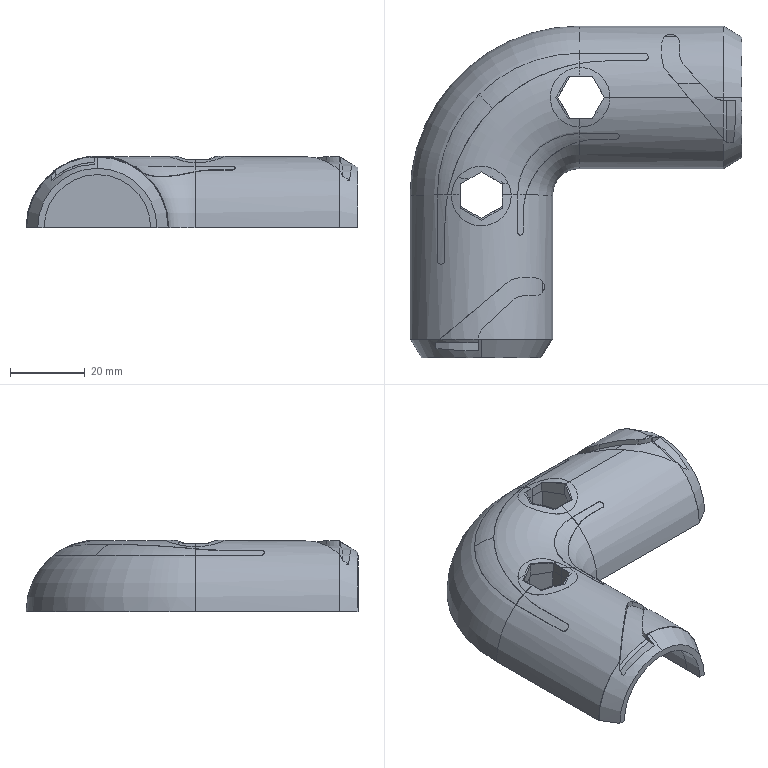Part | STEP file | GT-90D | 15 solids | 180 faces | box 89.055 x 89.077 x 19.235 mm | volume 46571 mm3 | plane 102 | cylinder 62 | torus 10 | cone 6 | commonest cylinder face diameters 38.27 x19 10 x8 28.6 x8 16 x7 87.726 x4 1.5 x3